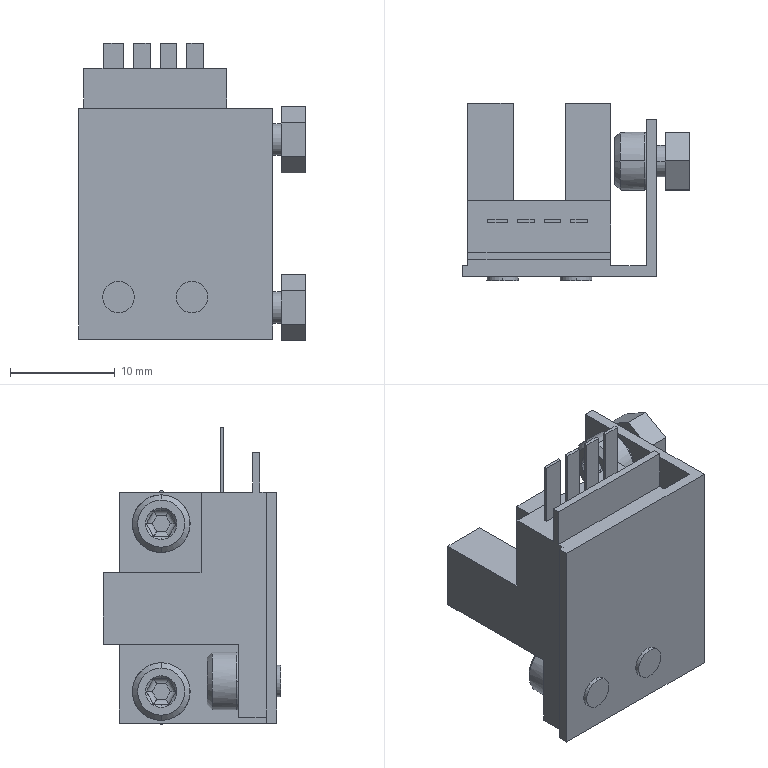Part | SolidWorks | features BaseBody 1 | 1 solid | 164 faces | box 21.6 x 16.9 x 28.375 mm | volume 3154 mm3 | plane 96 | cylinder 44 | cone 16 | spline 8 | commonest cylinder face diameters 1 x24 3 x12 5.5 x8